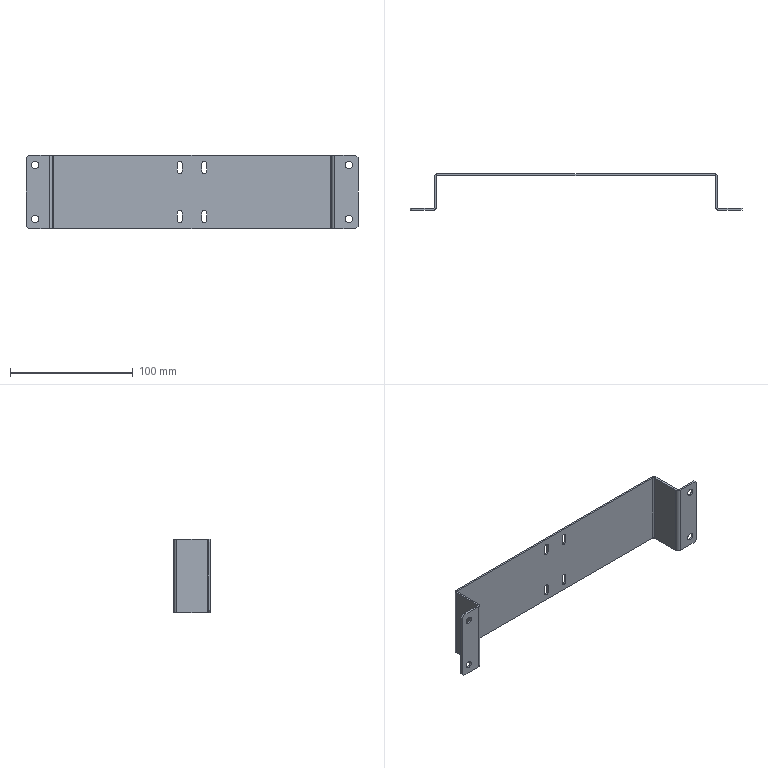Part | SolidWorks | features ICE 2, Chamfer 1, FlatPattern 1, HoleWzd 1, SMBaseFlange 1, SheetMetal 1 | 1 solid | 66 faces | box 270 x 29.5 x 60 mm | volume 28669 mm3 | plane 42 | cylinder 24 | commonest cylinder face diameters 4 x8 6 x8 2 x4 5 x4